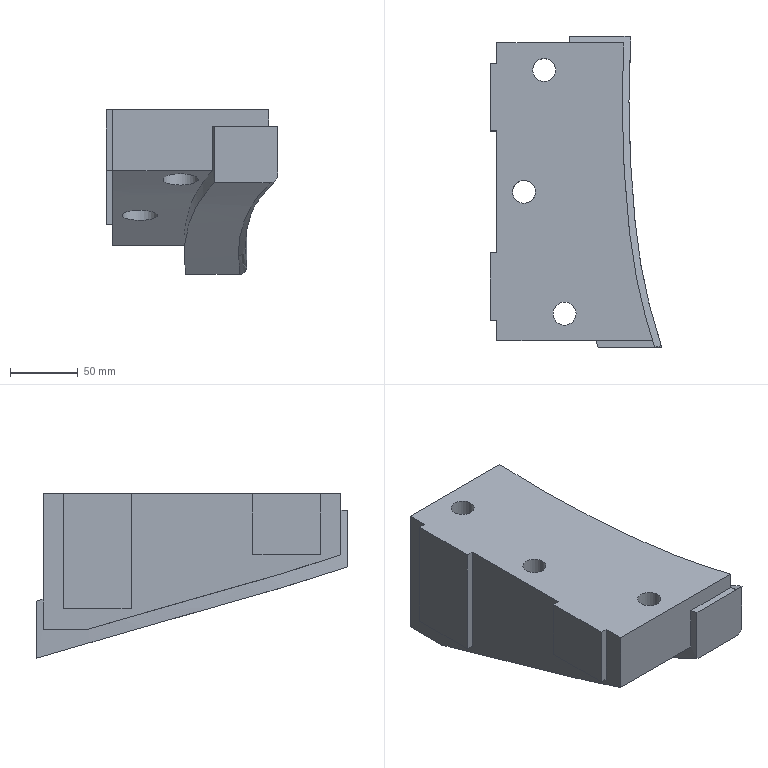Part | NX | features solid 2 | 1 solid | 33 faces | box 126.909 x 230 x 121.577 mm | volume 1737509 mm3 | plane 20 | spline 7 | cylinder 6 | commonest cylinder face diameters 17 x3 26 x3